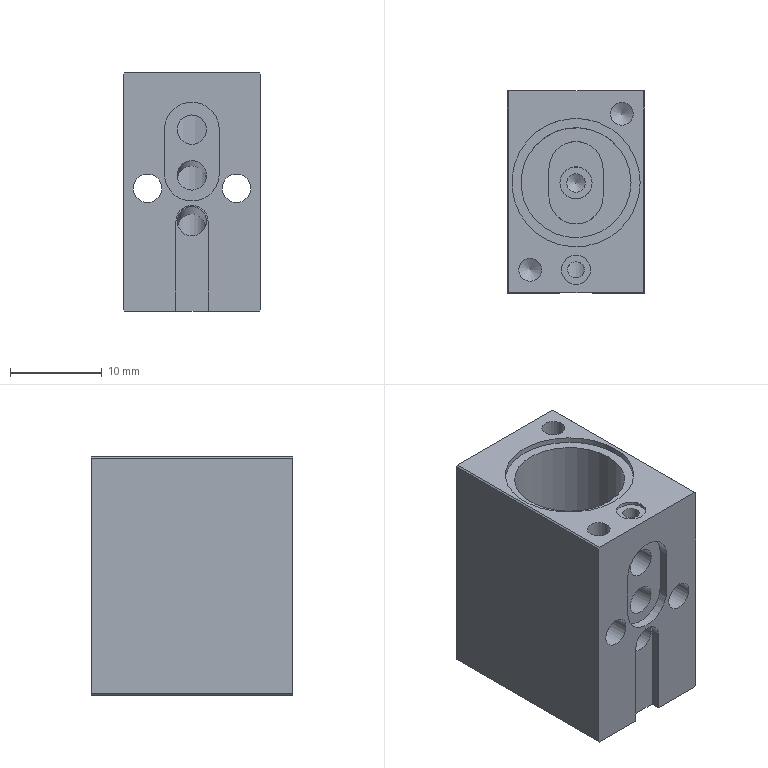NC program | NX | posted with a generic post | part box 15 x 22 x 26 mm
Lines 1766 to 2644 of 5185:
(CURVE_DRIVE , TOOL : D2R0.5)
N3458 T17 M6
N3460 G54
N3462 G17 G0 G90 X1.008 Y17.092 B0. C0. S4500 M3
N3464 G43 Z30. H17
N3466 Z2.74
N3468 G94 G1 Z-0.157 F1000.
N3470 X0.997 Y17.091 Z-0.299
N3472 X0.965 Z-0.438
N3474 X0.914 Y17.089 Z-0.572
N3476 X0.845 Y17.088 Z-0.696
N3478 X0.758 Y17.086 Z-0.81
N3480 X0.657 Y17.083 Z-0.91
N3482 X0.542 Y17.08 Z-0.994
N3484 X0.416 Y17.077 Z-1.062
N3486 X0.282 Y17.074 Z-1.11
N3488 X0.142 Y17.07 Z-1.139
N3490 X0. Y17.067 Z-1.148
N3492 X-0.249 Y17.061 Z-1.146
N3494 X-0.373 Y17.053 Z-1.149
N3496 X-0.497 Y17.043
N3498 X-0.743 Y17.012
N3500 X-0.989 Y16.97 Z-1.148
N3502 X-1.231 Y16.915 Z-1.15
N3504 X-1.471 Y16.849 Z-1.149
N3506 X-1.707 Y16.771
N3508 X-1.939 Y16.681 Z-1.148
N3510 X-2.166 Y16.581
N3512 X-2.389 Y16.469 Z-1.15
N3514 X-2.605 Y16.346 Z-1.149
N3516 X-2.815 Y16.213 Z-1.148
N3518 X-3.018 Y16.07 Z-1.147
N3520 X-3.214 Y15.917 Z-1.148
N3522 X-3.403 Y15.754 Z-1.15
N3524 X-3.583 Y15.583 Z-1.149
N3526 X-3.754 Y15.403 Z-1.147
N3528 X-3.837 Y15.31 Z-1.15
N3530 X-3.917 Y15.214 Z-1.147
N3532 X-4.07 Y15.018 Z-1.148
N3534 X-4.143 Y14.918 Z-1.147
N3536 X-4.213 Y14.815 Z-1.15
N3538 X-4.346 Y14.605 Z-1.148
N3540 X-4.409 Y14.498
N3542 X-4.469 Y14.389 Z-1.147
N3544 X-4.526 Y14.278 Z-1.15
N3546 X-4.581 Y14.166 Z-1.146
N3548 X-4.681 Y13.939 Z-1.148
N3550 X-4.727 Y13.824 Z-1.146
N3552 X-4.771 Y13.707 Z-1.15
N3554 X-4.811 Y13.589 Z-1.146
N3556 X-4.849 Y13.471 Z-1.147
N3558 X-4.915 Y13.231 Z-1.146
N3560 X-4.944 Y13.11 Z-1.149
N3562 X-4.97 Y12.989 Z-1.146
N3564 X-5.012 Y12.743 Z-1.147
N3566 X-5.043 Y12.497 Z-1.148
N3568 X-5.061 Y12.249 Z-1.146
N3570 X-5.067 Y12. Z-1.145
N3572 X-5.061 Y11.751 Z-1.146
N3574 X-5.043 Y11.503 Z-1.148
N3576 X-5.029 Y11.38 Z-1.145
N3578 X-5.012 Y11.257 Z-1.148
N3580 X-4.97 Y11.011 Z-1.146
N3582 X-4.944 Y10.89 Z-1.149
N3584 X-4.915 Y10.769 Z-1.146
N3586 X-4.849 Y10.529 Z-1.147
N3588 X-4.771 Y10.293 Z-1.15
N3590 X-4.727 Y10.176 Z-1.146
N3592 X-4.681 Y10.061 Z-1.148
N3594 X-4.581 Y9.834 Z-1.146
N3596 X-4.526 Y9.722 Z-1.15
N3598 X-4.469 Y9.611 Z-1.147
N3600 X-4.346 Y9.395 Z-1.148
N3602 X-4.213 Y9.185 Z-1.15
N3604 X-4.07 Y8.982 Z-1.148
N3606 X-3.995 Y8.883 Z-1.149
N3608 X-3.917 Y8.786 Z-1.147
N3610 X-3.754 Y8.597
N3612 X-3.583 Y8.417 Z-1.149
N3614 X-3.403 Y8.246 Z-1.15
N3616 X-3.214 Y8.083 Z-1.148
N3618 X-3.018 Y7.93 Z-1.147
N3620 X-2.815 Y7.787 Z-1.148
N3622 X-2.605 Y7.654 Z-1.149
N3624 X-2.389 Y7.531 Z-1.15
N3626 X-2.166 Y7.419 Z-1.148
N3628 X-1.939 Y7.319
N3630 X-1.707 Y7.229 Z-1.149
N3632 X-1.471 Y7.151
N3634 X-1.231 Y7.085 Z-1.15
N3636 X-0.989 Y7.03 Z-1.148
N3638 X-0.743 Y6.988 Z-1.149
N3640 X-0.497 Y6.957
N3642 X-0.249 Y6.939 Z-1.146
N3644 X0. Y6.933 Z-1.148
N3646 X0.249 Y6.939 Z-1.146
N3648 X0.373 Y6.947 Z-1.149
N3650 X0.497 Y6.957
N3652 X0.743 Y6.988
N3654 X0.989 Y7.03 Z-1.148
N3656 X1.231 Y7.085 Z-1.15
N3658 X1.471 Y7.151 Z-1.149
N3660 X1.707 Y7.229
N3662 X1.939 Y7.319 Z-1.148
N3664 X2.166 Y7.419
N3666 X2.389 Y7.531 Z-1.15
N3668 X2.605 Y7.654 Z-1.149
N3670 X2.815 Y7.787 Z-1.148
N3672 X3.018 Y7.93 Z-1.147
N3674 X3.214 Y8.083 Z-1.148
N3676 X3.403 Y8.246 Z-1.15
N3678 X3.583 Y8.417 Z-1.149
N3680 X3.754 Y8.597 Z-1.147
N3682 X3.837 Y8.69 Z-1.15
N3684 X3.917 Y8.786 Z-1.147
N3686 X4.07 Y8.982 Z-1.148
N3688 X4.143 Y9.082 Z-1.147
N3690 X4.213 Y9.185 Z-1.15
N3692 X4.346 Y9.395 Z-1.148
N3694 X4.409 Y9.502
N3696 X4.469 Y9.611 Z-1.147
N3698 X4.526 Y9.722 Z-1.15
N3700 X4.581 Y9.834 Z-1.146
N3702 X4.681 Y10.061 Z-1.148
N3704 X4.727 Y10.176 Z-1.146
N3706 X4.771 Y10.293 Z-1.15
N3708 X4.811 Y10.411 Z-1.146
N3710 X4.849 Y10.529 Z-1.147
N3712 X4.915 Y10.769 Z-1.146
N3714 X4.944 Y10.89 Z-1.149
N3716 X4.97 Y11.011 Z-1.146
N3718 X5.012 Y11.257 Z-1.147
N3720 X5.043 Y11.503 Z-1.148
N3722 X5.061 Y11.751 Z-1.146
N3724 X5.067 Y12. Z-1.145
N3726 X5.061 Y12.249 Z-1.146
N3728 X5.043 Y12.497 Z-1.148
N3730 X5.029 Y12.62 Z-1.145
N3732 X5.012 Y12.743 Z-1.148
N3734 X4.97 Y12.989 Z-1.146
N3736 X4.944 Y13.11 Z-1.149
N3738 X4.915 Y13.231 Z-1.146
N3740 X4.849 Y13.471 Z-1.147
N3742 X4.771 Y13.707 Z-1.15
N3744 X4.727 Y13.824 Z-1.146
N3746 X4.681 Y13.939 Z-1.148
N3748 X4.581 Y14.166 Z-1.146
N3750 X4.526 Y14.278 Z-1.15
N3752 X4.469 Y14.389 Z-1.147
N3754 X4.346 Y14.605 Z-1.148
N3756 X4.213 Y14.815 Z-1.15
N3758 X4.07 Y15.018 Z-1.148
N3760 X3.995 Y15.117 Z-1.149
N3762 X3.917 Y15.214 Z-1.147
N3764 X3.754 Y15.403
N3766 X3.583 Y15.583 Z-1.149
N3768 X3.403 Y15.754 Z-1.15
N3770 X3.214 Y15.917 Z-1.148
N3772 X3.018 Y16.07 Z-1.147
N3774 X2.815 Y16.213 Z-1.148
N3776 X2.605 Y16.346 Z-1.149
N3778 X2.389 Y16.469 Z-1.15
N3780 X2.166 Y16.581 Z-1.148
N3782 X1.939 Y16.681
N3784 X1.707 Y16.771 Z-1.149
N3786 X1.471 Y16.849
N3788 X1.231 Y16.915 Z-1.15
N3790 X0.989 Y16.97 Z-1.148
N3792 X0.743 Y17.012 Z-1.149
N3794 X0.497 Y17.043
N3796 X0.249 Y17.061 Z-1.146
N3798 X0. Y17.067 Z-1.148
N3800 X-0.249 Y17.061 Z-1.146
N3802 X-0.373 Y17.053 Z-1.148
N3804 X-0.497 Y17.043 Z-1.149
N3806 X-0.744 Y17.013 Z-1.148
N3808 X-0.989 Y16.97
N3810 X-1.231 Y16.916
N3812 X-1.471 Y16.85
N3814 X-1.707 Y16.772
N3816 X-1.824 Y16.728
N3818 X-1.939 Y16.682 Z-1.146
N3820 X-2.167 Y16.582
N3822 X-2.389 Y16.47 Z-1.147
N3824 X-2.606 Y16.347
N3826 X-2.712 Y16.282 Z-1.146
N3828 X-2.816 Y16.214
N3830 X-3.019 Y16.071 Z-1.144
N3832 X-3.216 Y15.918 Z-1.145
N3834 X-3.404 Y15.756 Z-1.146
N3836 X-3.495 Y15.671 Z-1.144
N3838 X-3.584 Y15.584 Z-1.146
N3840 X-3.756 Y15.404 Z-1.144
N3842 X-3.919 Y15.216 Z-1.143
N3844 X-4.072 Y15.02
N3846 X-4.145 Y14.919 Z-1.142
N3848 X-4.215 Y14.817 Z-1.145
N3850 X-4.349 Y14.606 Z-1.143
N3852 X-4.471 Y14.39 Z-1.141
N3854 X-4.529 Y14.28 Z-1.145
N3856 X-4.583 Y14.168 Z-1.141
N3858 X-4.684 Y13.94 Z-1.142
N3860 X-4.731 Y13.825 Z-1.14
N3862 X-4.774 Y13.708 Z-1.144
N3864 X-4.852 Y13.472 Z-1.141
N3866 X-4.919 Y13.232 Z-1.139
N3868 X-4.948 Y13.111 Z-1.143
N3870 X-4.973 Y12.989 Z-1.139
N3872 X-5.016 Y12.744 Z-1.141
N3874 X-5.033 Y12.621 Z-1.138
N3876 X-5.047 Y12.497 Z-1.141
N3878 X-5.065 Y12.249 Z-1.139
N3880 X-5.07 Y12.124 Z-1.14
N3882 X-5.071 Y12. Z-1.138
N3884 X-5.065 Y11.751
N3886 X-5.047 Y11.503 Z-1.14
N3888 X-5.034 Y11.379 Z-1.137
N3890 X-5.017 Y11.256 Z-1.14
N3892 X-4.974 Y11.011 Z-1.138
N3894 X-4.949 Y10.889 Z-1.141
N3896 X-4.92 Y10.768 Z-1.137
N3898 X-4.854 Y10.528 Z-1.138
N3900 X-4.776 Y10.291 Z-1.141
N3902 X-4.732 Y10.174 Z-1.137
N3904 X-4.686 Y10.059 Z-1.138
N3906 X-4.586 Y9.831 Z-1.137
N3908 X-4.531 Y9.719 Z-1.14
N3910 X-4.474 Y9.609 Z-1.137
N3912 X-4.351 Y9.392 Z-1.138
N3914 X-4.218 Y9.182 Z-1.14
N3916 X-4.075 Y8.978 Z-1.137
N3918 X-3.922 Y8.782 Z-1.136
N3920 X-3.759 Y8.593
N3922 X-3.587 Y8.413 Z-1.138
N3924 X-3.407 Y8.241
N3926 X-3.219 Y8.078 Z-1.136
N3928 X-3.023 Y7.925
N3930 X-2.819 Y7.781
N3932 X-2.609 Y7.648 Z-1.137
N3934 X-2.392 Y7.525
N3936 X-2.17 Y7.413 Z-1.135
N3938 X-1.942 Y7.312
N3940 X-1.71 Y7.222 Z-1.136
N3942 X-1.473 Y7.144
N3944 X-1.233 Y7.077
N3946 X-0.99 Y7.022 Z-1.134
N3948 X-0.745 Y6.98
N3950 X-0.497 Y6.949 Z-1.135
N3952 X-0.249 Y6.931 Z-1.132
N3954 X-0.125 Y6.926 Z-1.13
N3956 X0. Y6.924 Z-1.134
N3958 X0.125 Y6.926 Z-1.13
N3960 X0.249 Y6.93 Z-1.131
N3962 X0.373 Y6.938 Z-1.133
N3964 X0.498 Y6.949 Z-1.134
N3966 X0.745 Y6.979 Z-1.133
N3968 X0.99 Y7.021
N3970 X1.233 Y7.076 Z-1.134
N3972 X1.474 Y7.142 Z-1.133
N3974 X1.71 Y7.22
N3976 X1.943 Y7.31 Z-1.131
N3978 X2.171 Y7.411
N3980 X2.393 Y7.522 Z-1.132
N3982 X2.61 Y7.645
N3984 X2.821 Y7.778 Z-1.131
N3986 X3.025 Y7.922 Z-1.129
N3988 X3.221 Y8.075 Z-1.13
N3990 X3.41 Y8.238 Z-1.131
N3992 X3.501 Y8.322 Z-1.129
N3994 X3.591 Y8.409 Z-1.131
N3996 X3.763 Y8.59 Z-1.129
N3998 X3.925 Y8.778 Z-1.128
N4000 X4.079 Y8.975
N4002 X4.152 Y9.076 Z-1.127
N4004 X4.222 Y9.179 Z-1.13
N4006 X4.356 Y9.389 Z-1.128
N4008 X4.479 Y9.606 Z-1.126
N4010 X4.536 Y9.717 Z-1.13
N4012 X4.591 Y9.829 Z-1.126
N4014 X4.692 Y10.056 Z-1.127
N4016 X4.739 Y10.172 Z-1.125
N4018 X4.782 Y10.289 Z-1.129
N4020 X4.86 Y10.526 Z-1.126
N4022 X4.927 Y10.766 Z-1.124
N4024 X4.956 Y10.887 Z-1.128
N4026 X4.982 Y11.009 Z-1.124
N4028 X5.025 Y11.255 Z-1.126
N4030 X5.041 Y11.378 Z-1.123
N4032 X5.055 Y11.502 Z-1.126
N4034 X5.074 Y11.751 Z-1.124
N4036 X5.08 Y12. Z-1.123
N4038 X5.074 Y12.249
N4040 X5.056 Y12.498 Z-1.125
N4042 X5.042 Y12.622 Z-1.122
N4044 X5.025 Y12.745 Z-1.125
N4046 X4.983 Y12.991 Z-1.123
N4048 X4.957 Y13.113 Z-1.126
N4050 X4.928 Y13.234 Z-1.122
N4052 X4.862 Y13.475 Z-1.123
N4054 X4.784 Y13.712 Z-1.126
N4056 X4.741 Y13.829 Z-1.122
N4058 X4.694 Y13.944 Z-1.123
N4060 X4.593 Y14.172 Z-1.122
N4062 X4.539 Y14.285 Z-1.125
N4064 X4.481 Y14.395 Z-1.122
N4066 X4.359 Y14.612 Z-1.123
N4068 X4.225 Y14.823 Z-1.125
N4070 X4.082 Y15.027 Z-1.122
N4072 X3.928 Y15.224 Z-1.121
N4074 X3.766 Y15.413
N4076 X3.594 Y15.594 Z-1.123
N4078 X3.413 Y15.766
N4080 X3.224 Y15.929 Z-1.121
N4082 X3.028 Y16.082
N4084 X2.824 Y16.226
N4086 X2.613 Y16.36 Z-1.122
N4088 X2.396 Y16.483
N4090 X2.173 Y16.595 Z-1.12
N4092 X1.945 Y16.696
N4094 X1.713 Y16.786 Z-1.121
N4096 X1.476 Y16.865
N4098 X1.235 Y16.931
N4100 X0.992 Y16.986 Z-1.119
N4102 X0.746 Y17.029
N4104 X0.498 Y17.06 Z-1.12
N4106 X0.249 Y17.078 Z-1.117
N4108 X0.125 Y17.083 Z-1.115
N4110 X0. Y17.084 Z-1.119
N4112 X-0.125 Y17.083 Z-1.115
N4114 X-0.249 Y17.078 Z-1.116
N4116 X-0.374 Y17.071 Z-1.118
N4118 X-0.498 Y17.06 Z-1.119
N4120 X-0.746 Y17.03 Z-1.118
N4122 X-0.992 Y16.987
N4124 X-1.236 Y16.933 Z-1.119
N4126 X-1.476 Y16.866 Z-1.118
N4128 X-1.713 Y16.788
N4130 X-1.946 Y16.698 Z-1.116
N4132 X-2.174 Y16.597
N4134 X-2.397 Y16.485 Z-1.117
N4136 X-2.615 Y16.362
N4138 X-2.826 Y16.229 Z-1.116
N4140 X-3.03 Y16.085 Z-1.114
N4142 X-3.227 Y15.932 Z-1.115
N4144 X-3.416 Y15.769 Z-1.116
N4146 X-3.507 Y15.684 Z-1.114
N4148 X-3.597 Y15.597 Z-1.116
N4150 X-3.769 Y15.416 Z-1.114
N4152 X-3.932 Y15.227 Z-1.113
N4154 X-4.086 Y15.03
N4156 X-4.23 Y14.826 Z-1.115
N4158 X-4.363 Y14.615 Z-1.113
N4160 X-4.487 Y14.398 Z-1.111
N4162 X-4.544 Y14.287 Z-1.115
N4164 X-4.599 Y14.175 Z-1.111
N4166 X-4.7 Y13.947 Z-1.112
N4168 X-4.79 Y13.714 Z-1.114
N4170 X-4.869 Y13.477 Z-1.111
N4172 X-4.935 Y13.236 Z-1.109
N4174 X-4.964 Y13.115 Z-1.113
N4176 X-4.99 Y12.993 Z-1.109
N4178 X-5.033 Y12.747 Z-1.111
N4180 X-5.05 Y12.623 Z-1.108
N4182 X-5.064 Y12.499 Z-1.111
N4184 X-5.082 Y12.25 Z-1.109
N4186 X-5.089 Y12. Z-1.108
N4188 X-5.083 Y11.75
N4190 X-5.064 Y11.501 Z-1.11
N4192 X-5.051 Y11.377 Z-1.107
N4194 X-5.034 Y11.253 Z-1.11
N4196 X-4.991 Y11.007 Z-1.108
N4198 X-4.966 Y10.885 Z-1.11
N4200 X-4.937 Y10.763 Z-1.107
N4202 X-4.87 Y10.523 Z-1.108
N4204 X-4.792 Y10.285 Z-1.111
N4206 X-4.702 Y10.052 Z-1.108
N4208 X-4.601 Y9.824 Z-1.107
N4210 X-4.546 Y9.712 Z-1.11
N4212 X-4.489 Y9.601 Z-1.107
N4214 X-4.366 Y9.383 Z-1.108
N4216 X-4.232 Y9.172 Z-1.11
N4218 X-4.089 Y8.968 Z-1.107
N4220 X-3.935 Y8.771 Z-1.106
N4222 X-3.772 Y8.581
N4224 X-3.6 Y8.4 Z-1.108
N4226 X-3.419 Y8.228
N4228 X-3.23 Y8.065 Z-1.106
N4230 X-3.033 Y7.911
N4232 X-2.829 Y7.767
N4234 X-2.618 Y7.633 Z-1.107
N4236 X-2.4 Y7.51
N4238 X-2.177 Y7.397 Z-1.105
N4240 X-1.949 Y7.296
N4242 X-1.715 Y7.206 Z-1.106
N4244 X-1.478 Y7.127
N4246 X-1.237 Y7.06
N4248 X-0.993 Y7.005 Z-1.104
N4250 X-0.747 Y6.963
N4252 X-0.499 Y6.932 Z-1.105
N4254 X-0.25 Y6.913 Z-1.102
N4256 X-0.125 Y6.909 Z-1.1
N4258 X0. Y6.907 Z-1.104
N4260 X0.125 Y6.908 Z-1.1
N4262 X0.25 Y6.913 Z-1.101
N4264 X0.499 Y6.931 Z-1.104
N4266 X0.747 Y6.962 Z-1.103
N4268 X0.994 Y7.004
N4270 X1.238 Y7.059 Z-1.104
N4272 X1.359 Y7.091 Z-1.102
N4274 X1.479 Y7.126 Z-1.103
N4276 X1.716 Y7.204 Z-1.102
N4278 X1.949 Y7.294 Z-1.101
N4280 X2.178 Y7.395
N4282 X2.401 Y7.507 Z-1.102
N4284 X2.619 Y7.63
N4286 X2.83 Y7.764 Z-1.101
N4288 X3.035 Y7.908 Z-1.099
N4290 X3.232 Y8.062 Z-1.1
N4292 X3.422 Y8.225 Z-1.101
N4294 X3.513 Y8.31 Z-1.099
N4296 X3.603 Y8.397 Z-1.1
N4298 X3.775 Y8.578 Z-1.099
N4300 X3.939 Y8.768 Z-1.098
N4302 X4.093 Y8.965
N4304 X4.166 Y9.066 Z-1.097
N4306 X4.237 Y9.169 Z-1.1
N4308 X4.371 Y9.38 Z-1.098
N4310 X4.494 Y9.598 Z-1.096
N4312 X4.552 Y9.709 Z-1.1
N4314 X4.607 Y9.821 Z-1.096
N4316 X4.708 Y10.05 Z-1.097
N4318 X4.798 Y10.283 Z-1.099
N4320 X4.877 Y10.521 Z-1.096
N4322 X4.944 Y10.762 Z-1.094
N4324 X4.973 Y10.883 Z-1.098
N4326 X4.999 Y11.006 Z-1.094
N4328 X5.042 Y11.252 Z-1.096
N4330 X5.059 Y11.376 Z-1.093
N4332 X5.072 Y11.5 Z-1.096
N4334 X5.091 Y11.75 Z-1.094
N4336 X5.097 Y12. Z-1.093
N4338 X5.091 Y12.25
N4340 X5.073 Y12.5 Z-1.095
N4342 X5.059 Y12.624 Z-1.092
N4344 X5.043 Y12.748 Z-1.094
N4346 X5. Y12.995 Z-1.093
N4348 X4.974 Y13.117 Z-1.095
N4350 X4.945 Y13.239 Z-1.092
N4352 X4.879 Y13.48 Z-1.093
N4354 X4.8 Y13.718 Z-1.095
N4356 X4.71 Y13.951 Z-1.093
N4358 X4.609 Y14.18 Z-1.092
N4360 X4.554 Y14.292 Z-1.095
N4362 X4.497 Y14.403 Z-1.092
N4364 X4.373 Y14.621 Z-1.093
N4366 X4.24 Y14.833 Z-1.095
N4368 X4.096 Y15.038 Z-1.092
N4370 X3.942 Y15.235 Z-1.091
N4372 X3.778 Y15.425
N4374 X3.606 Y15.606 Z-1.093
N4376 X3.425 Y15.779
N4378 X3.235 Y15.942 Z-1.091
N4380 X3.038 Y16.096
N4382 X2.833 Y16.24
N4384 X2.622 Y16.375 Z-1.092
N4386 X2.404 Y16.498
N4388 X2.181 Y16.611 Z-1.09
N4390 X1.952 Y16.712
N4392 X1.718 Y16.803 Z-1.091
N4394 X1.481 Y16.881
N4396 X1.239 Y16.948
N4398 X0.995 Y17.003 Z-1.089
N4400 X0.749 Y17.046
N4402 X0.624 Y17.063 Z-1.09
N4404 X0.5 Y17.077
N4406 X0.25 Y17.095 Z-1.087
N4408 X0.125 Y17.1 Z-1.085
N4410 X0. Y17.102 Z-1.089
N4412 X-0.125 Y17.1 Z-1.085
N4414 X-0.25 Y17.096 Z-1.086
N4416 X-0.5 Y17.077 Z-1.089
N4418 X-0.749 Y17.047 Z-1.088
N4420 X-0.995 Y17.004
N4422 X-1.24 Y16.949 Z-1.089
N4424 X-1.361 Y16.918 Z-1.087
N4426 X-1.481 Y16.883 Z-1.088
N4428 X-1.719 Y16.804 Z-1.087
N4430 X-1.953 Y16.714 Z-1.086
N4432 X-2.182 Y16.613
N4434 X-2.406 Y16.5 Z-1.087
N4436 X-2.624 Y16.377
N4438 X-2.73 Y16.311 Z-1.085
N4440 X-2.835 Y16.243 Z-1.086
N4442 X-3.04 Y16.099 Z-1.084
N4444 X-3.238 Y15.945 Z-1.085
N4446 X-3.427 Y15.782 Z-1.086
N4448 X-3.519 Y15.696 Z-1.084
N4450 X-3.609 Y15.609 Z-1.085
N4452 X-3.782 Y15.428 Z-1.084
N4454 X-3.945 Y15.238 Z-1.083
N4456 X-4.1 Y15.041
N4458 X-4.173 Y14.939 Z-1.082
N4460 X-4.244 Y14.836 Z-1.085
N4462 X-4.378 Y14.624 Z-1.083
N4464 X-4.502 Y14.406 Z-1.081
N4466 X-4.56 Y14.295 Z-1.085
N4468 X-4.615 Y14.183 Z-1.081
N4470 X-4.716 Y13.954 Z-1.082
N4472 X-4.807 Y13.72 Z-1.084
N4474 X-4.885 Y13.482 Z-1.081
N4476 X-4.952 Y13.24 Z-1.079
N4478 X-4.981 Y13.119 Z-1.082
N4480 X-5.007 Y12.996 Z-1.079
N4482 X-5.05 Y12.749 Z-1.081
N4484 X-5.067 Y12.625 Z-1.078
N4486 X-5.081 Y12.5 Z-1.081
N4488 X-5.1 Y12.251 Z-1.079
N4490 X-5.106 Y12. Z-1.078
N4492 X-5.1 Y11.749
N4494 X-5.082 Y11.5 Z-1.08
N4496 X-5.068 Y11.375 Z-1.077
N4498 X-5.051 Y11.251 Z-1.079
N4500 X-5.008 Y11.004 Z-1.078
N4502 X-4.982 Y10.881 Z-1.08
N4504 X-4.954 Y10.759 Z-1.077
N4506 X-4.887 Y10.518 Z-1.078
N4508 X-4.808 Y10.28 Z-1.08
N4510 X-4.718 Y10.046 Z-1.078
N4512 X-4.617 Y9.816 Z-1.077
N4514 X-4.562 Y9.704 Z-1.08
N4516 X-4.504 Y9.592 Z-1.077
N4518 X-4.381 Y9.374 Z-1.078
N4520 X-4.247 Y9.162 Z-1.08
N4522 X-4.103 Y8.957 Z-1.077
N4524 X-3.948 Y8.76 Z-1.076
N4526 X-3.868 Y8.664 Z-1.079
N4528 X-3.785 Y8.57 Z-1.076
N4530 X-3.612 Y8.388 Z-1.078
N4532 X-3.43 Y8.215
N4534 X-3.241 Y8.051 Z-1.076
N4536 X-3.043 Y7.897
N4538 X-2.838 Y7.752
N4540 X-2.626 Y7.618 Z-1.077
N4542 X-2.408 Y7.494
N4544 X-2.184 Y7.381 Z-1.075
N4546 X-2.07 Y7.329 Z-1.076
N4548 X-1.955 Y7.28 Z-1.075
N4550 X-1.721 Y7.189
N4552 X-1.483 Y7.111 Z-1.076
N4554 X-1.242 Y7.044
N4556 X-0.997 Y6.988 Z-1.074
N4558 X-0.75 Y6.945
N4560 X-0.626 Y6.928 Z-1.075
N4562 X-0.501 Y6.915 Z-1.074
N4564 X-0.251 Y6.896 Z-1.072
N4566 X-0.125 Y6.891 Z-1.07
N4568 X0. Y6.89 Z-1.074
N4570 X0.125 Y6.891 Z-1.07
N4572 X0.251 Y6.896 Z-1.071
N4574 X0.501 Y6.914 Z-1.073
N4576 X0.75 Y6.945
N4578 X0.997 Y6.987
N4580 X1.242 Y7.042 Z-1.074
N4582 X1.363 Y7.074 Z-1.072
N4584 X1.484 Y7.109 Z-1.073
N4586 X1.722 Y7.188 Z-1.072
N4588 X1.956 Y7.278 Z-1.071
N4590 X2.185 Y7.379
N4592 X2.41 Y7.492 Z-1.072
N4594 X2.628 Y7.615
N4596 X2.735 Y7.681 Z-1.07
N4598 X2.84 Y7.75
N4600 X3.045 Y7.894 Z-1.069
N4602 X3.243 Y8.048 Z-1.07
N4604 X3.433 Y8.212 Z-1.071
N4606 X3.525 Y8.297 Z-1.069
N4608 X3.615 Y8.385 Z-1.07
N4610 X3.788 Y8.567 Z-1.069
N4612 X3.871 Y8.661 Z-1.071
N4614 X3.952 Y8.757 Z-1.068
N4616 X4.107 Y8.954
N4618 X4.18 Y9.056 Z-1.067
N4620 X4.251 Y9.159 Z-1.07
N4622 X4.386 Y9.371 Z-1.068
N4624 X4.509 Y9.59 Z-1.066
N4626 X4.567 Y9.701 Z-1.07
N4628 X4.622 Y9.814 Z-1.066
N4630 X4.724 Y10.043 Z-1.067
N4632 X4.815 Y10.277 Z-1.069
N4634 X4.856 Y10.396 Z-1.065
N4636 X4.894 Y10.516 Z-1.066
N4638 X4.961 Y10.757 Z-1.064
N4640 X4.99 Y10.88 Z-1.067
N4642 X5.016 Y11.002 Z-1.064
N4644 X5.059 Y11.25 Z-1.066
N4646 X5.076 Y11.374 Z-1.063
N4648 X5.09 Y11.499 Z-1.066
N4650 X5.108 Y11.749 Z-1.064
N4652 X5.115 Y12. Z-1.063
N4654 X5.109 Y12.251
N4656 X5.09 Y12.501 Z-1.065
N4658 X5.076 Y12.626 Z-1.062
N4660 X5.06 Y12.751 Z-1.064
N4662 X5.017 Y12.998 Z-1.063
N4664 X4.991 Y13.121 Z-1.065
N4666 X4.962 Y13.243 Z-1.062
N4668 X4.895 Y13.485 Z-1.063
N4670 X4.817 Y13.723 Z-1.065
N4672 X4.726 Y13.958 Z-1.063
N4674 X4.625 Y14.187 Z-1.062
N4676 X4.57 Y14.3 Z-1.065
N4678 X4.512 Y14.412 Z-1.062
N4680 X4.388 Y14.63 Z-1.063
N4682 X4.254 Y14.842 Z-1.065
N4684 X4.11 Y15.048 Z-1.062
N4686 X3.955 Y15.246 Z-1.061
N4688 X3.874 Y15.342 Z-1.064
N4690 X3.791 Y15.436 Z-1.061
N4692 X3.618 Y15.618 Z-1.062
N4694 X3.436 Y15.791 Z-1.063
N4696 X3.246 Y15.956 Z-1.061
N4698 X3.048 Y16.11
N4700 X2.843 Y16.255
N4702 X2.631 Y16.389 Z-1.062
N4704 X2.412 Y16.513
N4706 X2.188 Y16.626 Z-1.06
N4708 X2.074 Y16.679 Z-1.061
N4710 X1.959 Y16.728 Z-1.06
N4712 X1.724 Y16.819
N4714 X1.486 Y16.898 Z-1.061
N4716 X1.244 Y16.965
N4718 X0.999 Y17.02 Z-1.059
N4720 X0.751 Y17.063
N4722 X0.627 Y17.08 Z-1.06
N4724 X0.502 Y17.094 Z-1.059
N4726 X0.251 Y17.113 Z-1.057
N4728 X0.126 Y17.117 Z-1.055
N4730 X0. Y17.119 Z-1.059
N4732 X-0.126 Y17.117 Z-1.055
N4734 X-0.251 Y17.113 Z-1.056
N4736 X-0.502 Y17.095 Z-1.058
N4738 X-0.751 Y17.064
N4740 X-0.999 Y17.021
N4742 X-1.244 Y16.966 Z-1.059
N4744 X-1.365 Y16.934 Z-1.057
N4746 X-1.486 Y16.899 Z-1.058
N4748 X-1.725 Y16.821 Z-1.057
N4750 X-1.959 Y16.73 Z-1.056
N4752 X-2.189 Y16.629
N4754 X-2.414 Y16.516 Z-1.057
N4756 X-2.632 Y16.392
N4758 X-2.739 Y16.326 Z-1.055
N4760 X-2.845 Y16.258
N4762 X-3.05 Y16.113 Z-1.054
N4764 X-3.249 Y15.958 Z-1.055
N4766 X-3.439 Y15.794 Z-1.056
N4768 X-3.531 Y15.709 Z-1.054
N4770 X-3.621 Y15.621 Z-1.055
N4772 X-3.795 Y15.439 Z-1.053
N4774 X-3.878 Y15.345 Z-1.056
N4776 X-3.959 Y15.249 Z-1.053
N4778 X-4.114 Y15.051
N4780 X-4.259 Y14.845 Z-1.055
N4782 X-4.393 Y14.633 Z-1.053
N4784 X-4.517 Y14.414 Z-1.051
N4786 X-4.575 Y14.303 Z-1.055
N4788 X-4.63 Y14.19 Z-1.051
N4790 X-4.732 Y13.96 Z-1.052
N4792 X-4.823 Y13.726 Z-1.053
N4794 X-4.864 Y13.607 Z-1.05
N4796 X-4.902 Y13.487 Z-1.051
N4798 X-4.969 Y13.245 Z-1.049
N4800 X-4.998 Y13.122 Z-1.052
N4802 X-5.024 Y12.999 Z-1.049
N4804 X-5.067 Y12.752 Z-1.051
N4806 X-5.084 Y12.627 Z-1.048
N4808 X-5.098 Y12.502 Z-1.051
N4810 X-5.117 Y12.251 Z-1.049
N4812 X-5.123 Y12. Z-1.048
N4814 X-5.117 Y11.749
N4816 X-5.099 Y11.498 Z-1.05
N4818 X-5.085 Y11.373 Z-1.047
N4820 X-5.068 Y11.248 Z-1.049
N4822 X-5.025 Y11. Z-1.048
N4824 X-4.999 Y10.877 Z-1.05
N4826 X-4.97 Y10.755 Z-1.047
N4828 X-4.903 Y10.513 Z-1.048
N4830 X-4.825 Y10.274 Z-1.05
N4832 X-4.734 Y10.039 Z-1.048
N4834 X-4.632 Y9.809 Z-1.047
N4836 X-4.577 Y9.696 Z-1.05
N4838 X-4.52 Y9.584 Z-1.047
N4840 X-4.396 Y9.365 Z-1.048
N4842 X-4.261 Y9.153 Z-1.05
N4844 X-4.116 Y8.947 Z-1.047
N4846 X-3.962 Y8.749 Z-1.046
N4848 X-3.881 Y8.652 Z-1.049
N4850 X-3.798 Y8.558 Z-1.046
N4852 X-3.624 Y8.376 Z-1.047
N4854 X-3.442 Y8.202 Z-1.048
N4856 X-3.252 Y8.038 Z-1.046
N4858 X-3.053 Y7.883
N4860 X-2.848 Y7.738
N4862 X-2.635 Y7.603 Z-1.047
N4864 X-2.417 Y7.479
N4866 X-2.192 Y7.366 Z-1.045
N4868 X-1.962 Y7.264
N4870 X-1.727 Y7.173
N4872 X-1.488 Y7.094 Z-1.046
N4874 X-1.246 Y7.027
N4876 X-1.123 Y6.998 Z-1.044
N4878 X-1. Y6.971
N4880 X-0.752 Y6.928
N4882 X-0.503 Y6.897
N4884 X-0.252 Y6.879 Z-1.042
N4886 X-0.126 Y6.874 Z-1.04
N4888 X0. Y6.872 Z-1.044
N4890 X0.126 Y6.874 Z-1.04
N4892 X0.252 Y6.878 Z-1.041
N4894 X0.503 Y6.897 Z-1.043
N4896 X0.752 Y6.927
N4898 X1. Y6.97
N4900 X1.246 Y7.025 Z-1.044
N4902 X1.489 Y7.092 Z-1.043
N4904 X1.728 Y7.171 Z-1.041
N4906 X1.963 Y7.262
N4908 X2.193 Y7.364
N4910 X2.418 Y7.477 Z-1.042
N4912 X2.637 Y7.601 Z-1.041
N4914 X2.744 Y7.667 Z-1.04
N4916 X2.85 Y7.735
N4918 X3.056 Y7.88 Z-1.039
N4920 X3.254 Y8.035 Z-1.04
N4922 X3.445 Y8.199 Z-1.041
N4924 X3.627 Y8.373 Z-1.04
N4926 X3.801 Y8.555 Z-1.038
N4928 X3.884 Y8.649 Z-1.041
N4930 X3.966 Y8.746 Z-1.038
N4932 X4.121 Y8.944
N4934 X4.266 Y9.15 Z-1.04
N4936 X4.401 Y9.362 Z-1.038
N4938 X4.464 Y9.471
N4940 X4.525 Y9.581 Z-1.036
N4942 X4.583 Y9.693 Z-1.039
N4944 X4.638 Y9.806 Z-1.036
N4946 X4.74 Y10.037 Z-1.037
N4948 X4.831 Y10.271 Z-1.038
N4950 X4.872 Y10.39 Z-1.035
N4952 X4.91 Y10.511 Z-1.036
N4954 X4.977 Y10.753 Z-1.034
N4956 X5.007 Y10.876 Z-1.037
N4958 X5.033 Y10.999 Z-1.034
N4960 X5.076 Y11.247 Z-1.036
N4962 X5.093 Y11.372 Z-1.033
N4964 X5.107 Y11.497 Z-1.036
N4966 X5.126 Y11.748 Z-1.034
N4968 X5.132 Y12. Z-1.033
N4970 X5.126 Y12.252
N4972 X5.107 Y12.503 Z-1.035
N4974 X5.094 Y12.628 Z-1.032
N4976 X5.077 Y12.753 Z-1.034
N4978 X5.034 Y13.001 Z-1.033
N4980 X5.008 Y13.125 Z-1.035
N4982 X4.979 Y13.247 Z-1.032
N4984 X4.912 Y13.49 Z-1.033
N4986 X4.833 Y13.729 Z-1.035
N4988 X4.742 Y13.964 Z-1.033
N4990 X4.64 Y14.195 Z-1.032
N4992 X4.585 Y14.308 Z-1.035
N4994 X4.527 Y14.42 Z-1.032
N4996 X4.403 Y14.639 Z-1.033
N4998 X4.268 Y14.852 Z-1.035
N5000 X4.123 Y15.058 Z-1.032
N5002 X4.047 Y15.158
N5004 X3.969 Y15.257 Z-1.031
N5006 X3.887 Y15.353 Z-1.034
N5008 X3.804 Y15.448 Z-1.031
N5010 X3.63 Y15.63 Z-1.032
N5012 X3.448 Y15.804 Z-1.033
N5014 X3.257 Y15.969 Z-1.031
N5016 X3.059 Y16.124
N5018 X2.853 Y16.269 Z-1.03
N5020 X2.64 Y16.404 Z-1.031
N5022 X2.421 Y16.529 Z-1.032
N5024 X2.196 Y16.642 Z-1.03
N5026 X1.965 Y16.744
N5028 X1.73 Y16.835
N5030 X1.491 Y16.914 Z-1.031
N5032 X1.248 Y16.982
N5034 X1.125 Y17.011 Z-1.029
N5036 X1.002 Y17.037
N5038 X0.754 Y17.08
N5040 X0.503 Y17.111
N5042 X0.252 Y17.13 Z-1.027
N5044 X0.126 Y17.135 Z-1.025
N5046 X0. Y17.136 Z-1.029
N5048 X-0.126 Y17.135 Z-1.025
N5050 X-0.252 Y17.13 Z-1.026
N5052 X-0.503 Y17.112 Z-1.028
N5054 X-0.754 Y17.081 Z-1.027
N5056 X-1.002 Y17.038 Z-1.028
N5058 X-1.248 Y16.983 Z-1.029
N5060 X-1.491 Y16.916 Z-1.028
N5062 X-1.731 Y16.837 Z-1.026
N5064 X-1.849 Y16.793 Z-1.028
N5066 X-1.966 Y16.746 Z-1.026
N5068 X-2.197 Y16.644
N5070 X-2.31 Y16.589 Z-1.025
N5072 X-2.422 Y16.531 Z-1.027
N5074 X-2.641 Y16.407 Z-1.026
N5076 X-2.854 Y16.272 Z-1.025
N5078 X-3.061 Y16.127 Z-1.024
N5080 X-3.26 Y15.972 Z-1.025
N5082 X-3.451 Y15.807 Z-1.026
N5084 X-3.633 Y15.633 Z-1.024
N5086 X-3.807 Y15.451 Z-1.023
N5088 X-3.891 Y15.356 Z-1.026
N5090 X-3.972 Y15.26 Z-1.023
N5092 X-4.128 Y15.061
N5094 X-4.273 Y14.855 Z-1.025
N5096 X-4.408 Y14.642 Z-1.023
N5098 X-4.472 Y14.533
N5100 X-4.532 Y14.423 Z-1.021
N5102 X-4.591 Y14.311 Z-1.024
N5104 X-4.646 Y14.197 Z-1.021
N5106 X-4.748 Y13.967 Z-1.022
N5108 X-4.839 Y13.731 Z-1.023
N5110 X-4.88 Y13.612 Z-1.02
N5112 X-4.918 Y13.492 Z-1.021
N5114 X-4.986 Y13.249 Z-1.019
N5116 X-5.015 Y13.126 Z-1.022
N5118 X-5.041 Y13.003 Z-1.019
N5120 X-5.085 Y12.754 Z-1.021
N5122 X-5.102 Y12.629 Z-1.018
N5124 X-5.116 Y12.504 Z-1.021
N5126 X-5.134 Y12.252 Z-1.019
N5128 X-5.141 Y12. Z-1.018
N5130 X-5.135 Y11.748
N5132 X-5.116 Y11.496 Z-1.02
N5134 X-5.102 Y11.371 Z-1.017
N5136 X-5.085 Y11.246 Z-1.019
N5138 X-5.042 Y10.997 Z-1.018
N5140 X-5.016 Y10.874 Z-1.02
N5142 X-4.987 Y10.751 Z-1.017
N5144 X-4.92 Y10.508 Z-1.018
N5146 X-4.841 Y10.268 Z-1.02
N5148 X-4.75 Y10.032 Z-1.018
N5150 X-4.648 Y9.802 Z-1.017
N5152 X-4.593 Y9.688 Z-1.02
N5154 X-4.535 Y9.576 Z-1.017
N5156 X-4.411 Y9.356
N5158 X-4.276 Y9.143 Z-1.02
N5160 X-4.13 Y8.937 Z-1.017
N5162 X-4.054 Y8.836
N5164 X-3.975 Y8.738 Z-1.016
N5166 X-3.894 Y8.641 Z-1.019
N5168 X-3.81 Y8.546 Z-1.016
N5170 X-3.636 Y8.364 Z-1.017
N5172 X-3.454 Y8.189 Z-1.018
N5174 X-3.263 Y8.024 Z-1.016
N5176 X-3.064 Y7.869
N5178 X-2.857 Y7.723 Z-1.015
N5180 X-2.644 Y7.588 Z-1.016
N5182 X-2.425 Y7.464 Z-1.017
N5184 X-2.199 Y7.35 Z-1.015
N5186 X-1.968 Y7.248
N5188 X-1.733 Y7.157 Z-1.014
N5190 X-1.493 Y7.077 Z-1.015
N5192 X-1.25 Y7.01 Z-1.016
N5194 X-1.127 Y6.981 Z-1.014
N5196 X-1.004 Y6.954
N5198 X-0.755 Y6.911
N5200 X-0.504 Y6.88 Z-1.013
N5202 X-0.252 Y6.861 Z-1.012
N5204 X-0.126 Y6.857 Z-1.01
N5206 X0. Y6.855 Z-1.014
N5208 X0.126 Y6.857 Z-1.01